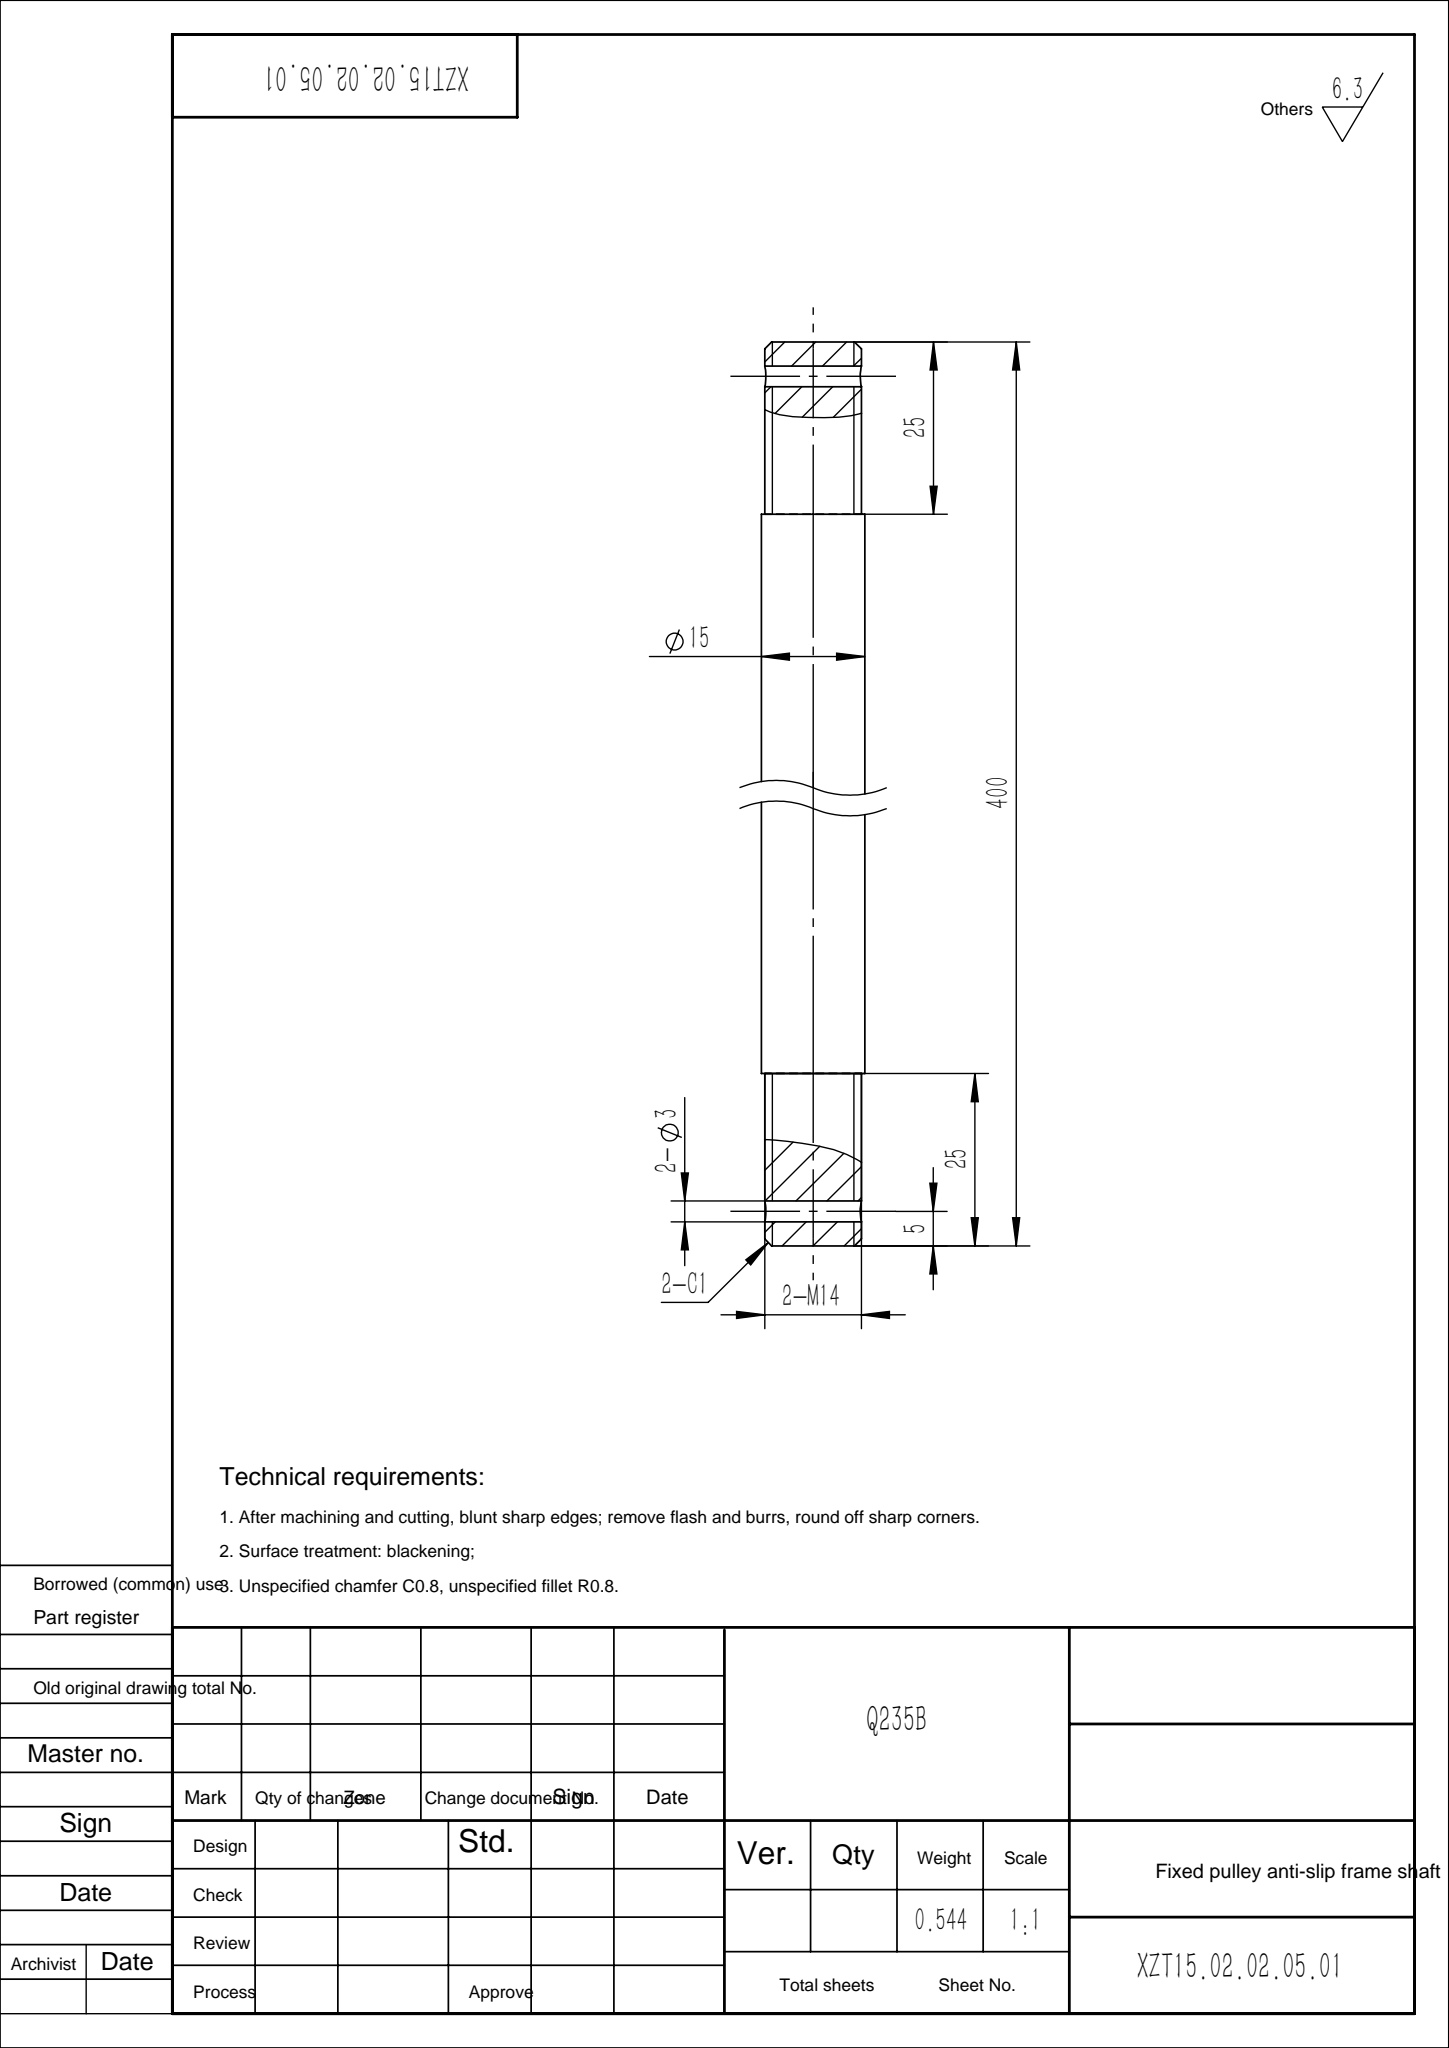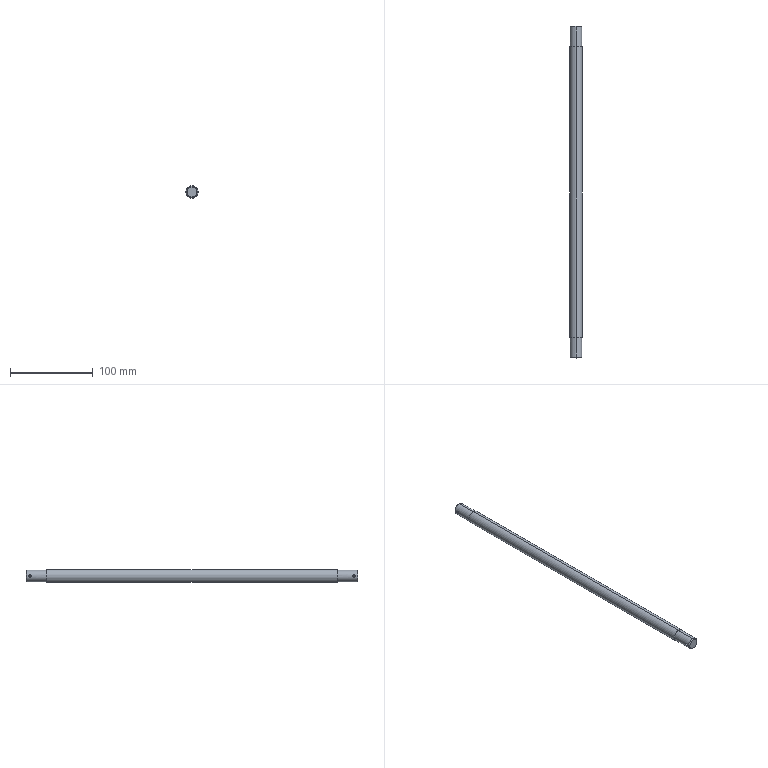Part | SolidWorks | features Chamfer 1, ICE 1, Revolution 1 | 1 solid | 18 faces | box 15 x 400 x 15 mm | volume 69308 mm3 | cylinder 10 | cone 4 | plane 4 | commonest cylinder face diameters 3 x4 14 x4 15 x2
STEP:
#1=CARTESIAN_POINT('',(-6.837,5.,1.5));
#2=VERTEX_POINT('',#1);
#3=CARTESIAN_POINT('',(-6.837,5.,-1.5));
#4=VERTEX_POINT('',#3);
#5=CARTESIAN_POINT('',(-6.837,5.,1.5));
#6=CARTESIAN_POINT('',(-6.837,4.804,1.5));
#7=CARTESIAN_POINT('',(-6.846,4.606,1.46));
#8=CARTESIAN_POINT('',(-6.877,4.245,1.311));
#9=CARTESIAN_POINT('',(-6.898,4.078,1.199));
#10=CARTESIAN_POINT('',(-6.93,3.871,0.9922));
#11=CARTESIAN_POINT('',(-6.94,3.808,0.9153));
#12=CARTESIAN_POINT('',(-6.96,3.699,0.753));
#13=CARTESIAN_POINT('',(-6.969,3.653,0.667));
#14=CARTESIAN_POINT('',(-6.991,3.539,0.3938));
#15=CARTESIAN_POINT('',(-7.,3.5,0.1987));
#16=CARTESIAN_POINT('',(-7.,3.5,-0.09833));
#17=CARTESIAN_POINT('',(-6.998,3.51,-0.1959));
#18=CARTESIAN_POINT('',(-6.99,3.548,-0.3882));
#19=CARTESIAN_POINT('',(-6.984,3.577,-0.4839));
#20=CARTESIAN_POINT('',(-6.961,3.689,-0.7556));
#21=CARTESIAN_POINT('',(-6.94,3.801,-0.9222));
#22=CARTESIAN_POINT('',(-6.898,4.076,-1.198));
#23=CARTESIAN_POINT('',(-6.877,4.243,-1.31));
#24=CARTESIAN_POINT('',(-6.846,4.604,-1.46));
#25=CARTESIAN_POINT('',(-6.837,4.801,-1.5));
#26=CARTESIAN_POINT('',(-6.837,5.,-1.5));
#27=B_SPLINE_CURVE_WITH_KNOTS('',3,(#5,#6,#7,#8,#9,#10,#11,#12,#13,#14,#15,#16,#17,#18,#19,#20,#21,#22,#23,#24,#25,#26),.UNSPECIFIED.,.F.,.F.,(4,2,2,2,2,2,2,2,2,2,4),(0.004703,0.005291,0.005879,0.006173,0.006467,0.007054,0.007348,0.007642,0.00823,0.008818,0.009405),.UNSPECIFIED.);
#28=EDGE_CURVE('',#2,#4,#27,.T.);
#29=ORIENTED_EDGE('',*,*,#28,.F.);
#30=CARTESIAN_POINT('',(6.837,5.,1.5));
#31=VERTEX_POINT('',#30);
#32=CARTESIAN_POINT('',(-7.5,5.,1.5));
#33=DIRECTION('',(1.,0.,0.));
#34=VECTOR('',#33,1000.);
#35=LINE('',#32,#34);
#36=EDGE_CURVE('',#2,#31,#35,.T.);
#37=ORIENTED_EDGE('',*,*,#36,.T.);
#38=CARTESIAN_POINT('',(6.837,5.,-1.5));
#39=VERTEX_POINT('',#38);
#40=CARTESIAN_POINT('',(6.837,5.,-1.5));
#41=CARTESIAN_POINT('',(6.837,4.901,-1.5));
#42=CARTESIAN_POINT('',(6.84,4.803,-1.49));
#43=CARTESIAN_POINT('',(6.848,4.611,-1.452));
#44=CARTESIAN_POINT('',(6.854,4.515,-1.423));
#45=CARTESIAN_POINT('',(6.869,4.334,-1.348));
#46=CARTESIAN_POINT('',(6.878,4.248,-1.301));
#47=CARTESIAN_POINT('',(6.898,4.085,-1.193));
#48=CARTESIAN_POINT('',(6.909,4.008,-1.129));
#49=CARTESIAN_POINT('',(6.94,3.801,-0.9225));
#50=CARTESIAN_POINT('',(6.961,3.69,-0.7555));
#51=CARTESIAN_POINT('',(6.991,3.54,-0.3947));
#52=CARTESIAN_POINT('',(7.,3.5,-0.1969));
#53=CARTESIAN_POINT('',(7.,3.5,0.09757));
#54=CARTESIAN_POINT('',(6.998,3.51,0.1973));
#55=CARTESIAN_POINT('',(6.99,3.548,0.3899));
#56=CARTESIAN_POINT('',(6.984,3.577,0.4836));
#57=CARTESIAN_POINT('',(6.961,3.69,0.7565));
#58=CARTESIAN_POINT('',(6.941,3.8,0.9216));
#59=CARTESIAN_POINT('',(6.908,4.009,1.13));
#60=CARTESIAN_POINT('',(6.898,4.085,1.192));
#61=CARTESIAN_POINT('',(6.878,4.247,1.301));
#62=CARTESIAN_POINT('',(6.869,4.335,1.348));
#63=CARTESIAN_POINT('',(6.854,4.516,1.423));
#64=CARTESIAN_POINT('',(6.848,4.609,1.452));
#65=CARTESIAN_POINT('',(6.84,4.802,1.49));
#66=CARTESIAN_POINT('',(6.837,4.902,1.5));
#67=CARTESIAN_POINT('',(6.837,5.,1.5));
#68=B_SPLINE_CURVE_WITH_KNOTS('',3,(#40,#41,#42,#43,#44,#45,#46,#47,#48,#49,#50,#51,#52,#53,#54,#55,#56,#57,#58,#59,#60,#61,#62,#63,#64,#65,#66,#67),.UNSPECIFIED.,.F.,.F.,(4,2,2,2,2,2,2,2,2,2,2,2,2,4),(0.,0.000294,0.0005879,0.0008819,0.001176,0.001764,0.002352,0.002646,0.00294,0.003527,0.003821,0.004115,0.004409,0.004703),.UNSPECIFIED.);
#69=EDGE_CURVE('',#39,#31,#68,.T.);
#70=ORIENTED_EDGE('',*,*,#69,.F.);
#71=CARTESIAN_POINT('',(-7.5,5.,-1.5));
#72=DIRECTION('',(1.,0.,0.));
#73=VECTOR('',#72,1000.);
#74=LINE('',#71,#73);
#75=EDGE_CURVE('',#4,#39,#74,.T.);
#76=ORIENTED_EDGE('',*,*,#75,.F.);
#77=EDGE_LOOP('',(#29,#37,#70,#76));
#78=FACE_OUTER_BOUND('',#77,.T.);
#79=CARTESIAN_POINT('',(-7.5,5.,0.));
#80=DIRECTION('',(1.,0.,0.));
#81=DIRECTION('',(0.,0.,-1.));
#82=AXIS2_PLACEMENT_3D('',#79,#80,#81);
#83=CYLINDRICAL_SURFACE('',#82,1.5);
#84=ADVANCED_FACE('',(#78),#83,.F.);
#85=CARTESIAN_POINT('',(-6.837,395.,1.5));
#86=VERTEX_POINT('',#85);
#87=CARTESIAN_POINT('',(-6.837,395.,-1.5));
#88=VERTEX_POINT('',#87);
#89=CARTESIAN_POINT('',(-6.837,395.,1.5));
#90=CARTESIAN_POINT('',(-6.837,394.804,1.5));
#91=CARTESIAN_POINT('',(-6.846,394.606,1.46));
#92=CARTESIAN_POINT('',(-6.877,394.245,1.311));
#93=CARTESIAN_POINT('',(-6.898,394.078,1.199));
#94=CARTESIAN_POINT('',(-6.93,393.871,0.9922));
#95=CARTESIAN_POINT('',(-6.94,393.808,0.9153));
#96=CARTESIAN_POINT('',(-6.96,393.699,0.753));
#97=CARTESIAN_POINT('',(-6.969,393.653,0.667));
#98=CARTESIAN_POINT('',(-6.991,393.539,0.3938));
#99=CARTESIAN_POINT('',(-7.,393.5,0.1987));
#100=CARTESIAN_POINT('',(-7.,393.5,-0.09833));
#101=CARTESIAN_POINT('',(-6.998,393.51,-0.1959));
#102=CARTESIAN_POINT('',(-6.99,393.548,-0.3882));
#103=CARTESIAN_POINT('',(-6.984,393.577,-0.4839));
#104=CARTESIAN_POINT('',(-6.961,393.689,-0.7556));
#105=CARTESIAN_POINT('',(-6.94,393.801,-0.9222));
#106=CARTESIAN_POINT('',(-6.898,394.076,-1.198));
#107=CARTESIAN_POINT('',(-6.877,394.243,-1.31));
#108=CARTESIAN_POINT('',(-6.846,394.604,-1.46));
#109=CARTESIAN_POINT('',(-6.837,394.801,-1.5));
#110=CARTESIAN_POINT('',(-6.837,395.,-1.5));
#111=B_SPLINE_CURVE_WITH_KNOTS('',3,(#89,#90,#91,#92,#93,#94,#95,#96,#97,#98,#99,#100,#101,#102,#103,#104,#105,#106,#107,#108,#109,#110),.UNSPECIFIED.,.F.,.F.,(4,2,2,2,2,2,2,2,2,2,4),(0.004703,0.005291,0.005879,0.006173,0.006467,0.007054,0.007348,0.007642,0.00823,0.008818,0.009405),.UNSPECIFIED.);
#112=EDGE_CURVE('',#86,#88,#111,.T.);
#113=ORIENTED_EDGE('',*,*,#112,.F.);
#114=CARTESIAN_POINT('',(6.837,395.,1.5));
#115=VERTEX_POINT('',#114);
#116=CARTESIAN_POINT('',(-7.5,395.,1.5));
#117=DIRECTION('',(1.,0.,0.));
#118=VECTOR('',#117,1000.);
#119=LINE('',#116,#118);
#120=EDGE_CURVE('',#86,#115,#119,.T.);
#121=ORIENTED_EDGE('',*,*,#120,.T.);
#122=CARTESIAN_POINT('',(6.837,395.,-1.5));
#123=VERTEX_POINT('',#122);
#124=CARTESIAN_POINT('',(6.837,395.,-1.5));
#125=CARTESIAN_POINT('',(6.837,394.901,-1.5));
#126=CARTESIAN_POINT('',(6.84,394.803,-1.49));
#127=CARTESIAN_POINT('',(6.848,394.611,-1.452));
#128=CARTESIAN_POINT('',(6.854,394.515,-1.423));
#129=CARTESIAN_POINT('',(6.869,394.334,-1.348));
#130=CARTESIAN_POINT('',(6.878,394.248,-1.301));
#131=CARTESIAN_POINT('',(6.898,394.085,-1.193));
#132=CARTESIAN_POINT('',(6.909,394.008,-1.129));
#133=CARTESIAN_POINT('',(6.94,393.801,-0.9225));
#134=CARTESIAN_POINT('',(6.961,393.69,-0.7555));
#135=CARTESIAN_POINT('',(6.991,393.54,-0.3947));
#136=CARTESIAN_POINT('',(7.,393.5,-0.1969));
#137=CARTESIAN_POINT('',(7.,393.5,0.09757));
#138=CARTESIAN_POINT('',(6.998,393.51,0.1973));
#139=CARTESIAN_POINT('',(6.99,393.548,0.3899));
#140=CARTESIAN_POINT('',(6.984,393.577,0.4836));
#141=CARTESIAN_POINT('',(6.961,393.69,0.7565));
#142=CARTESIAN_POINT('',(6.941,393.8,0.9216));
#143=CARTESIAN_POINT('',(6.908,394.009,1.13));
#144=CARTESIAN_POINT('',(6.898,394.085,1.192));
#145=CARTESIAN_POINT('',(6.878,394.247,1.301));
#146=CARTESIAN_POINT('',(6.869,394.335,1.348));
#147=CARTESIAN_POINT('',(6.854,394.516,1.423));
#148=CARTESIAN_POINT('',(6.848,394.609,1.452));
#149=CARTESIAN_POINT('',(6.84,394.802,1.49));
#150=CARTESIAN_POINT('',(6.837,394.902,1.5));
#151=CARTESIAN_POINT('',(6.837,395.,1.5));
#152=B_SPLINE_CURVE_WITH_KNOTS('',3,(#124,#125,#126,#127,#128,#129,#130,#131,#132,#133,#134,#135,#136,#137,#138,#139,#140,#141,#142,#143,#144,#145,#146,#147,#148,#149,#150,#151),.UNSPECIFIED.,.F.,.F.,(4,2,2,2,2,2,2,2,2,2,2,2,2,4),(0.,0.000294,0.0005879,0.0008819,0.001176,0.001764,0.002352,0.002646,0.00294,0.003527,0.003821,0.004115,0.004409,0.004703),.UNSPECIFIED.);
#153=EDGE_CURVE('',#123,#115,#152,.T.);
#154=ORIENTED_EDGE('',*,*,#153,.F.);
#155=CARTESIAN_POINT('',(-7.5,395.,-1.5));
#156=DIRECTION('',(1.,0.,0.));
#157=VECTOR('',#156,1000.);
#158=LINE('',#155,#157);
#159=EDGE_CURVE('',#88,#123,#158,.T.);
#160=ORIENTED_EDGE('',*,*,#159,.F.);
#161=EDGE_LOOP('',(#113,#121,#154,#160));
#162=FACE_OUTER_BOUND('',#161,.T.);
#163=CARTESIAN_POINT('',(-7.5,395.,0.));
#164=DIRECTION('',(1.,0.,0.));
#165=DIRECTION('',(0.,0.,-1.));
#166=AXIS2_PLACEMENT_3D('',#163,#164,#165);
#167=CYLINDRICAL_SURFACE('',#166,1.5);
#168=ADVANCED_FACE('',(#162),#167,.F.);
#169=CARTESIAN_POINT('',(0.,400.,6.));
#170=VERTEX_POINT('',#169);
#171=CARTESIAN_POINT('',(0.,400.,-6.));
#172=VERTEX_POINT('',#171);
#173=CARTESIAN_POINT('',(0.,400.,0.));
#174=DIRECTION('',(0.,1.,0.));
#175=DIRECTION('',(0.,0.,-1.));
#176=AXIS2_PLACEMENT_3D('',#173,#174,#175);
#177=CIRCLE('',#176,6.);
#178=EDGE_CURVE('',#170,#172,#177,.T.);
#179=ORIENTED_EDGE('',*,*,#178,.F.);
#180=CARTESIAN_POINT('',(0.,399.,7.));
#181=VERTEX_POINT('',#180);
#182=CARTESIAN_POINT('',(0.,400.,6.));
#183=DIRECTION('',(0.,-0.7071,0.7071));
#184=VECTOR('',#183,1000.);
#185=LINE('',#182,#184);
#186=EDGE_CURVE('',#170,#181,#185,.T.);
#187=ORIENTED_EDGE('',*,*,#186,.T.);
#188=CARTESIAN_POINT('',(0.,399.,-7.));
#189=VERTEX_POINT('',#188);
#190=CARTESIAN_POINT('',(0.,399.,0.));
#191=DIRECTION('',(0.,-1.,0.));
#192=DIRECTION('',(0.,0.,-1.));
#193=AXIS2_PLACEMENT_3D('',#190,#191,#192);
#194=CIRCLE('',#193,7.);
#195=EDGE_CURVE('',#189,#181,#194,.T.);
#196=ORIENTED_EDGE('',*,*,#195,.F.);
#197=CARTESIAN_POINT('',(0.,400.,-6.));
#198=DIRECTION('',(0.,-0.7071,-0.7071));
#199=VECTOR('',#198,1000.);
#200=LINE('',#197,#199);
#201=EDGE_CURVE('',#172,#189,#200,.T.);
#202=ORIENTED_EDGE('',*,*,#201,.F.);
#203=EDGE_LOOP('',(#179,#187,#196,#202));
#204=FACE_OUTER_BOUND('',#203,.T.);
#205=CARTESIAN_POINT('',(0.,400.,0.));
#206=DIRECTION('',(0.,-1.,0.));
#207=DIRECTION('',(0.,0.,-1.));
#208=AXIS2_PLACEMENT_3D('',#205,#206,#207);
#209=CONICAL_SURFACE('',#208,6.,0.7854);
#210=ADVANCED_FACE('',(#204),#209,.T.);
#211=CARTESIAN_POINT('',(0.,0.,-6.));
#212=VERTEX_POINT('',#211);
#213=CARTESIAN_POINT('',(0.,0.,6.));
#214=VERTEX_POINT('',#213);
#215=CARTESIAN_POINT('',(0.,0.,0.));
#216=DIRECTION('',(0.,-1.,0.));
#217=DIRECTION('',(0.,0.,1.));
#218=AXIS2_PLACEMENT_3D('',#215,#216,#217);
#219=CIRCLE('',#218,6.);
#220=EDGE_CURVE('',#212,#214,#219,.T.);
#221=ORIENTED_EDGE('',*,*,#220,.F.);
#222=CARTESIAN_POINT('',(0.,1.,-7.));
#223=VERTEX_POINT('',#222);
#224=CARTESIAN_POINT('',(0.,1.,-7.));
#225=DIRECTION('',(0.,0.7071,-0.7071));
#226=VECTOR('',#225,1000.);
#227=LINE('',#224,#226);
#228=EDGE_CURVE('',#212,#223,#227,.T.);
#229=ORIENTED_EDGE('',*,*,#228,.T.);
#230=CARTESIAN_POINT('',(0.,1.,7.));
#231=VERTEX_POINT('',#230);
#232=CARTESIAN_POINT('',(0.,1.,0.));
#233=DIRECTION('',(0.,1.,0.));
#234=DIRECTION('',(0.,0.,1.));
#235=AXIS2_PLACEMENT_3D('',#232,#233,#234);
#236=CIRCLE('',#235,7.);
#237=EDGE_CURVE('',#231,#223,#236,.T.);
#238=ORIENTED_EDGE('',*,*,#237,.F.);
#239=CARTESIAN_POINT('',(0.,1.,7.));
#240=DIRECTION('',(0.,0.7071,0.7071));
#241=VECTOR('',#240,1000.);
#242=LINE('',#239,#241);
#243=EDGE_CURVE('',#214,#231,#242,.T.);
#244=ORIENTED_EDGE('',*,*,#243,.F.);
#245=EDGE_LOOP('',(#221,#229,#238,#244));
#246=FACE_OUTER_BOUND('',#245,.T.);
#247=CARTESIAN_POINT('',(0.,1.,0.));
#248=DIRECTION('',(0.,1.,0.));
#249=DIRECTION('',(0.,0.,1.));
#250=AXIS2_PLACEMENT_3D('',#247,#248,#249);
#251=CONICAL_SURFACE('',#250,7.,0.7854);
#252=ADVANCED_FACE('',(#246),#251,.T.);
#253=ORIENTED_EDGE('',*,*,#153,.T.);
#254=CARTESIAN_POINT('',(6.837,395.,1.5));
#255=CARTESIAN_POINT('',(6.837,395.196,1.5));
#256=CARTESIAN_POINT('',(6.846,395.394,1.46));
#257=CARTESIAN_POINT('',(6.877,395.755,1.311));
#258=CARTESIAN_POINT('',(6.898,395.922,1.199));
#259=CARTESIAN_POINT('',(6.93,396.129,0.9922));
#260=CARTESIAN_POINT('',(6.94,396.192,0.9153));
#261=CARTESIAN_POINT('',(6.96,396.301,0.753));
#262=CARTESIAN_POINT('',(6.969,396.347,0.667));
#263=CARTESIAN_POINT('',(6.991,396.461,0.3938));
#264=CARTESIAN_POINT('',(7.,396.5,0.1987));
#265=CARTESIAN_POINT('',(7.,396.5,-0.09833));
#266=CARTESIAN_POINT('',(6.998,396.49,-0.1959));
#267=CARTESIAN_POINT('',(6.99,396.452,-0.3882));
#268=CARTESIAN_POINT('',(6.984,396.423,-0.4839));
#269=CARTESIAN_POINT('',(6.961,396.311,-0.7556));
#270=CARTESIAN_POINT('',(6.94,396.199,-0.9222));
#271=CARTESIAN_POINT('',(6.898,395.924,-1.198));
#272=CARTESIAN_POINT('',(6.877,395.757,-1.31));
#273=CARTESIAN_POINT('',(6.846,395.396,-1.46));
#274=CARTESIAN_POINT('',(6.837,395.199,-1.5));
#275=CARTESIAN_POINT('',(6.837,395.,-1.5));
#276=B_SPLINE_CURVE_WITH_KNOTS('',3,(#254,#255,#256,#257,#258,#259,#260,#261,#262,#263,#264,#265,#266,#267,#268,#269,#270,#271,#272,#273,#274,#275),.UNSPECIFIED.,.F.,.F.,(4,2,2,2,2,2,2,2,2,2,4),(0.004703,0.005291,0.005879,0.006173,0.006467,0.007054,0.007348,0.007642,0.00823,0.008818,0.009405),.UNSPECIFIED.);
#277=EDGE_CURVE('',#115,#123,#276,.T.);
#278=ORIENTED_EDGE('',*,*,#277,.T.);
#279=EDGE_LOOP('',(#253,#278));
#280=FACE_BOUND('',#279,.T.);
#281=CARTESIAN_POINT('',(0.,375.,7.));
#282=VERTEX_POINT('',#281);
#283=CARTESIAN_POINT('',(0.,375.,-7.));
#284=VERTEX_POINT('',#283);
#285=CARTESIAN_POINT('',(0.,375.,0.));
#286=DIRECTION('',(0.,1.,0.));
#287=DIRECTION('',(0.,0.,1.));
#288=AXIS2_PLACEMENT_3D('',#285,#286,#287);
#289=CIRCLE('',#288,7.);
#290=EDGE_CURVE('',#282,#284,#289,.T.);
#291=ORIENTED_EDGE('',*,*,#290,.T.);
#292=CARTESIAN_POINT('',(0.,0.,-7.));
#293=DIRECTION('',(0.,1.,0.));
#294=VECTOR('',#293,1000.);
#295=LINE('',#292,#294);
#296=EDGE_CURVE('',#284,#189,#295,.T.);
#297=ORIENTED_EDGE('',*,*,#296,.T.);
#298=ORIENTED_EDGE('',*,*,#195,.T.);
#299=CARTESIAN_POINT('',(0.,0.,7.));
#300=DIRECTION('',(0.,1.,0.));
#301=VECTOR('',#300,1000.);
#302=LINE('',#299,#301);
#303=EDGE_CURVE('',#282,#181,#302,.T.);
#304=ORIENTED_EDGE('',*,*,#303,.F.);
#305=EDGE_LOOP('',(#291,#297,#298,#304));
#306=FACE_OUTER_BOUND('',#305,.T.);
#307=CARTESIAN_POINT('',(0.,0.,0.));
#308=DIRECTION('',(0.,1.,0.));
#309=DIRECTION('',(0.,0.,1.));
#310=AXIS2_PLACEMENT_3D('',#307,#308,#309);
#311=CYLINDRICAL_SURFACE('',#310,7.);
#312=ADVANCED_FACE('',(#280,#306),#311,.T.);
#313=CARTESIAN_POINT('',(0.,25.,7.5));
#314=VERTEX_POINT('',#313);
#315=CARTESIAN_POINT('',(0.,25.,-7.5));
#316=VERTEX_POINT('',#315);
#317=CARTESIAN_POINT('',(0.,25.,0.));
#318=DIRECTION('',(0.,1.,0.));
#319=DIRECTION('',(0.,0.,1.));
#320=AXIS2_PLACEMENT_3D('',#317,#318,#319);
#321=CIRCLE('',#320,7.5);
#322=EDGE_CURVE('',#314,#316,#321,.T.);
#323=ORIENTED_EDGE('',*,*,#322,.T.);
#324=CARTESIAN_POINT('',(0.,375.,-7.5));
#325=VERTEX_POINT('',#324);
#326=CARTESIAN_POINT('',(0.,0.,-7.5));
#327=DIRECTION('',(0.,1.,0.));
#328=VECTOR('',#327,1000.);
#329=LINE('',#326,#328);
#330=EDGE_CURVE('',#316,#325,#329,.T.);
#331=ORIENTED_EDGE('',*,*,#330,.T.);
#332=CARTESIAN_POINT('',(0.,375.,7.5));
#333=VERTEX_POINT('',#332);
#334=CARTESIAN_POINT('',(0.,375.,0.));
#335=DIRECTION('',(0.,1.,0.));
#336=DIRECTION('',(0.,0.,1.));
#337=AXIS2_PLACEMENT_3D('',#334,#335,#336);
#338=CIRCLE('',#337,7.5);
#339=EDGE_CURVE('',#333,#325,#338,.T.);
#340=ORIENTED_EDGE('',*,*,#339,.F.);
#341=CARTESIAN_POINT('',(0.,0.,7.5));
#342=DIRECTION('',(0.,1.,0.));
#343=VECTOR('',#342,1000.);
#344=LINE('',#341,#343);
#345=EDGE_CURVE('',#314,#333,#344,.T.);
#346=ORIENTED_EDGE('',*,*,#345,.F.);
#347=EDGE_LOOP('',(#323,#331,#340,#346));
#348=FACE_OUTER_BOUND('',#347,.T.);
#349=CARTESIAN_POINT('',(0.,0.,0.));
#350=DIRECTION('',(0.,1.,0.));
#351=DIRECTION('',(0.,0.,1.));
#352=AXIS2_PLACEMENT_3D('',#349,#350,#351);
#353=CYLINDRICAL_SURFACE('',#352,7.5);
#354=ADVANCED_FACE('',(#348),#353,.T.);
#355=ORIENTED_EDGE('',*,*,#69,.T.);
#356=CARTESIAN_POINT('',(6.837,5.,1.5));
#357=CARTESIAN_POINT('',(6.837,5.196,1.5));
#358=CARTESIAN_POINT('',(6.846,5.394,1.46));
#359=CARTESIAN_POINT('',(6.877,5.755,1.311));
#360=CARTESIAN_POINT('',(6.898,5.922,1.199));
#361=CARTESIAN_POINT('',(6.93,6.129,0.9922));
#362=CARTESIAN_POINT('',(6.94,6.192,0.9153));
#363=CARTESIAN_POINT('',(6.96,6.301,0.753));
#364=CARTESIAN_POINT('',(6.969,6.347,0.667));
#365=CARTESIAN_POINT('',(6.991,6.461,0.3938));
#366=CARTESIAN_POINT('',(7.,6.5,0.1987));
#367=CARTESIAN_POINT('',(7.,6.5,-0.09833));
#368=CARTESIAN_POINT('',(6.998,6.49,-0.1959));
#369=CARTESIAN_POINT('',(6.99,6.452,-0.3882));
#370=CARTESIAN_POINT('',(6.984,6.423,-0.4839));
#371=CARTESIAN_POINT('',(6.961,6.311,-0.7556));
#372=CARTESIAN_POINT('',(6.94,6.199,-0.9222));
#373=CARTESIAN_POINT('',(6.898,5.924,-1.198));
#374=CARTESIAN_POINT('',(6.877,5.757,-1.31));
#375=CARTESIAN_POINT('',(6.846,5.396,-1.46));
#376=CARTESIAN_POINT('',(6.837,5.199,-1.5));
#377=CARTESIAN_POINT('',(6.837,5.,-1.5));
#378=B_SPLINE_CURVE_WITH_KNOTS('',3,(#356,#357,#358,#359,#360,#361,#362,#363,#364,#365,#366,#367,#368,#369,#370,#371,#372,#373,#374,#375,#376,#377),.UNSPECIFIED.,.F.,.F.,(4,2,2,2,2,2,2,2,2,2,4),(0.004703,0.005291,0.005879,0.006173,0.006467,0.007054,0.007348,0.007642,0.00823,0.008818,0.009405),.UNSPECIFIED.);
#379=EDGE_CURVE('',#31,#39,#378,.T.);
#380=ORIENTED_EDGE('',*,*,#379,.T.);
#381=EDGE_LOOP('',(#355,#380));
#382=FACE_BOUND('',#381,.T.);
#383=ORIENTED_EDGE('',*,*,#237,.T.);
#384=CARTESIAN_POINT('',(0.,25.,-7.));
#385=VERTEX_POINT('',#384);
#386=CARTESIAN_POINT('',(0.,0.,-7.));
#387=DIRECTION('',(0.,1.,0.));
#388=VECTOR('',#387,1000.);
#389=LINE('',#386,#388);
#390=EDGE_CURVE('',#223,#385,#389,.T.);
#391=ORIENTED_EDGE('',*,*,#390,.T.);
#392=CARTESIAN_POINT('',(0.,25.,7.));
#393=VERTEX_POINT('',#392);
#394=CARTESIAN_POINT('',(0.,25.,0.));
#395=DIRECTION('',(0.,1.,0.));
#396=DIRECTION('',(0.,0.,1.));
#397=AXIS2_PLACEMENT_3D('',#394,#395,#396);
#398=CIRCLE('',#397,7.);
#399=EDGE_CURVE('',#393,#385,#398,.T.);
#400=ORIENTED_EDGE('',*,*,#399,.F.);
#401=CARTESIAN_POINT('',(0.,0.,7.));
#402=DIRECTION('',(0.,1.,0.));
#403=VECTOR('',#402,1000.);
#404=LINE('',#401,#403);
#405=EDGE_CURVE('',#231,#393,#404,.T.);
#406=ORIENTED_EDGE('',*,*,#405,.F.);
#407=EDGE_LOOP('',(#383,#391,#400,#406));
#408=FACE_OUTER_BOUND('',#407,.T.);
#409=CARTESIAN_POINT('',(0.,0.,0.));
#410=DIRECTION('',(0.,1.,0.));
#411=DIRECTION('',(0.,0.,1.));
#412=AXIS2_PLACEMENT_3D('',#409,#410,#411);
#413=CYLINDRICAL_SURFACE('',#412,7.);
#414=ADVANCED_FACE('',(#382,#408),#413,.T.);
#415=CARTESIAN_POINT('',(0.,0.,0.));
#416=DIRECTION('',(0.,-1.,0.));
#417=DIRECTION('',(0.,0.,1.));
#418=AXIS2_PLACEMENT_3D('',#415,#416,#417);
#419=CIRCLE('',#418,6.);
#420=EDGE_CURVE('',#214,#212,#419,.T.);
#421=ORIENTED_EDGE('',*,*,#420,.T.);
#422=ORIENTED_EDGE('',*,*,#220,.T.);
#423=EDGE_LOOP('',(#421,#422));
#424=FACE_OUTER_BOUND('',#423,.T.);
#425=CARTESIAN_POINT('',(0.,0.,0.));
#426=DIRECTION('',(0.,1.,0.));
#427=DIRECTION('',(0.,0.,1.));
#428=AXIS2_PLACEMENT_3D('',#425,#426,#427);
#429=PLANE('',#428);
#430=ADVANCED_FACE('',(#424),#429,.F.);
#431=ORIENTED_EDGE('',*,*,#390,.F.);
#432=CARTESIAN_POINT('',(0.,1.,0.));
#433=DIRECTION('',(0.,1.,0.));
#434=DIRECTION('',(0.,0.,1.));
#435=AXIS2_PLACEMENT_3D('',#432,#433,#434);
#436=CIRCLE('',#435,7.);
#437=EDGE_CURVE('',#223,#231,#436,.T.);
#438=ORIENTED_EDGE('',*,*,#437,.T.);
#439=ORIENTED_EDGE('',*,*,#405,.T.);
#440=CARTESIAN_POINT('',(0.,25.,0.));
#441=DIRECTION('',(0.,1.,0.));
#442=DIRECTION('',(0.,0.,1.));
#443=AXIS2_PLACEMENT_3D('',#440,#441,#442);
#444=CIRCLE('',#443,7.);
#445=EDGE_CURVE('',#385,#393,#444,.T.);
#446=ORIENTED_EDGE('',*,*,#445,.F.);
#447=EDGE_LOOP('',(#431,#438,#439,#446));
#448=FACE_OUTER_BOUND('',#447,.T.);
#449=CARTESIAN_POINT('',(-6.837,5.,-1.5));
#450=CARTESIAN_POINT('',(-6.837,5.099,-1.5));
#451=CARTESIAN_POINT('',(-6.84,5.197,-1.49));
#452=CARTESIAN_POINT('',(-6.848,5.389,-1.452));
#453=CARTESIAN_POINT('',(-6.854,5.485,-1.423));
#454=CARTESIAN_POINT('',(-6.869,5.666,-1.348));
#455=CARTESIAN_POINT('',(-6.878,5.752,-1.301));
#456=CARTESIAN_POINT('',(-6.898,5.915,-1.193));
#457=CARTESIAN_POINT('',(-6.909,5.992,-1.129));
#458=CARTESIAN_POINT('',(-6.94,6.199,-0.9225));
#459=CARTESIAN_POINT('',(-6.961,6.31,-0.7555));
#460=CARTESIAN_POINT('',(-6.991,6.46,-0.3947));
#461=CARTESIAN_POINT('',(-7.,6.5,-0.1969));
#462=CARTESIAN_POINT('',(-7.,6.5,0.09757));
#463=CARTESIAN_POINT('',(-6.998,6.49,0.1973));
#464=CARTESIAN_POINT('',(-6.99,6.452,0.3899));
#465=CARTESIAN_POINT('',(-6.984,6.423,0.4836));
#466=CARTESIAN_POINT('',(-6.961,6.31,0.7565));
#467=CARTESIAN_POINT('',(-6.941,6.2,0.9216));
#468=CARTESIAN_POINT('',(-6.908,5.991,1.13));
#469=CARTESIAN_POINT('',(-6.898,5.915,1.192));
#470=CARTESIAN_POINT('',(-6.878,5.753,1.301));
#471=CARTESIAN_POINT('',(-6.869,5.665,1.348));
#472=CARTESIAN_POINT('',(-6.854,5.484,1.423));
#473=CARTESIAN_POINT('',(-6.848,5.391,1.452));
#474=CARTESIAN_POINT('',(-6.84,5.198,1.49));
#475=CARTESIAN_POINT('',(-6.837,5.098,1.5));
#476=CARTESIAN_POINT('',(-6.837,5.,1.5));
#477=B_SPLINE_CURVE_WITH_KNOTS('',3,(#449,#450,#451,#452,#453,#454,#455,#456,#457,#458,#459,#460,#461,#462,#463,#464,#465,#466,#467,#468,#469,#470,#471,#472,#473,#474,#475,#476),.UNSPECIFIED.,.F.,.F.,(4,2,2,2,2,2,2,2,2,2,2,2,2,4),(0.,0.000294,0.0005879,0.0008819,0.001176,0.001764,0.002352,0.002646,0.00294,0.003527,0.003821,0.004115,0.004409,0.004703),.UNSPECIFIED.);
#478=EDGE_CURVE('',#4,#2,#477,.T.);
#479=ORIENTED_EDGE('',*,*,#478,.T.);
#480=ORIENTED_EDGE('',*,*,#28,.T.);
#481=EDGE_LOOP('',(#479,#480));
#482=FACE_BOUND('',#481,.T.);
#483=CARTESIAN_POINT('',(0.,0.,0.));
#484=DIRECTION('',(0.,1.,0.));
#485=DIRECTION('',(0.,0.,1.));
#486=AXIS2_PLACEMENT_3D('',#483,#484,#485);
#487=CYLINDRICAL_SURFACE('',#486,7.);
#488=ADVANCED_FACE('',(#448,#482),#487,.T.);
#489=ORIENTED_EDGE('',*,*,#322,.F.);
#490=CARTESIAN_POINT('',(0.,25.,0.));
#491=DIRECTION('',(0.,1.,0.));
#492=DIRECTION('',(0.,0.,1.));
#493=AXIS2_PLACEMENT_3D('',#490,#491,#492);
#494=CIRCLE('',#493,7.5);
#495=EDGE_CURVE('',#316,#314,#494,.T.);
#496=ORIENTED_EDGE('',*,*,#495,.F.);
#497=EDGE_LOOP('',(#489,#496));
#498=FACE_OUTER_BOUND('',#497,.T.);
#499=ORIENTED_EDGE('',*,*,#399,.T.);
#500=ORIENTED_EDGE('',*,*,#445,.T.);
#501=EDGE_LOOP('',(#499,#500));
#502=FACE_BOUND('',#501,.T.);
#503=CARTESIAN_POINT('',(7.,25.,0.));
#504=DIRECTION('',(0.,1.,0.));
#505=DIRECTION('',(0.,0.,1.));
#506=AXIS2_PLACEMENT_3D('',#503,#504,#505);
#507=PLANE('',#506);
#508=ADVANCED_FACE('',(#498,#502),#507,.F.);
#509=ORIENTED_EDGE('',*,*,#330,.F.);
#510=ORIENTED_EDGE('',*,*,#495,.T.);
#511=ORIENTED_EDGE('',*,*,#345,.T.);
#512=CARTESIAN_POINT('',(0.,375.,0.));
#513=DIRECTION('',(0.,1.,0.));
#514=DIRECTION('',(0.,0.,1.));
#515=AXIS2_PLACEMENT_3D('',#512,#513,#514);
#516=CIRCLE('',#515,7.5);
#517=EDGE_CURVE('',#325,#333,#516,.T.);
#518=ORIENTED_EDGE('',*,*,#517,.F.);
#519=EDGE_LOOP('',(#509,#510,#511,#518));
#520=FACE_OUTER_BOUND('',#519,.T.);
#521=CARTESIAN_POINT('',(0.,0.,0.));
#522=DIRECTION('',(0.,1.,0.));
#523=DIRECTION('',(0.,0.,1.));
#524=AXIS2_PLACEMENT_3D('',#521,#522,#523);
#525=CYLINDRICAL_SURFACE('',#524,7.5);
#526=ADVANCED_FACE('',(#520),#525,.T.);
#527=ORIENTED_EDGE('',*,*,#290,.F.);
#528=CARTESIAN_POINT('',(0.,375.,0.));
#529=DIRECTION('',(0.,1.,0.));
#530=DIRECTION('',(0.,0.,1.));
#531=AXIS2_PLACEMENT_3D('',#528,#529,#530);
#532=CIRCLE('',#531,7.);
#533=EDGE_CURVE('',#284,#282,#532,.T.);
#534=ORIENTED_EDGE('',*,*,#533,.F.);
#535=EDGE_LOOP('',(#527,#534));
#536=FACE_BOUND('',#535,.T.);
#537=ORIENTED_EDGE('',*,*,#339,.T.);
#538=ORIENTED_EDGE('',*,*,#517,.T.);
#539=EDGE_LOOP('',(#537,#538));
#540=FACE_OUTER_BOUND('',#539,.T.);
#541=CARTESIAN_POINT('',(7.5,375.,0.));
#542=DIRECTION('',(0.,-1.,0.));
#543=DIRECTION('',(0.,0.,-1.));
#544=AXIS2_PLACEMENT_3D('',#541,#542,#543);
#545=PLANE('',#544);
#546=ADVANCED_FACE('',(#536,#540),#545,.F.);
#547=ORIENTED_EDGE('',*,*,#296,.F.);
#548=ORIENTED_EDGE('',*,*,#533,.T.);
#549=ORIENTED_EDGE('',*,*,#303,.T.);
#550=CARTESIAN_POINT('',(0.,399.,0.));
#551=DIRECTION('',(0.,-1.,0.));
#552=DIRECTION('',(0.,0.,-1.));
#553=AXIS2_PLACEMENT_3D('',#550,#551,#552);
#554=CIRCLE('',#553,7.);
#555=EDGE_CURVE('',#181,#189,#554,.T.);
#556=ORIENTED_EDGE('',*,*,#555,.T.);
#557=EDGE_LOOP('',(#547,#548,#549,#556));
#558=FACE_OUTER_BOUND('',#557,.T.);
#559=CARTESIAN_POINT('',(-6.837,395.,-1.5));
#560=CARTESIAN_POINT('',(-6.837,395.099,-1.5));
#561=CARTESIAN_POINT('',(-6.84,395.197,-1.49));
#562=CARTESIAN_POINT('',(-6.848,395.389,-1.452));
#563=CARTESIAN_POINT('',(-6.854,395.485,-1.423));
#564=CARTESIAN_POINT('',(-6.869,395.666,-1.348));
#565=CARTESIAN_POINT('',(-6.878,395.752,-1.301));
#566=CARTESIAN_POINT('',(-6.898,395.915,-1.193));
#567=CARTESIAN_POINT('',(-6.909,395.992,-1.129));
#568=CARTESIAN_POINT('',(-6.94,396.199,-0.9225));
#569=CARTESIAN_POINT('',(-6.961,396.31,-0.7555));
#570=CARTESIAN_POINT('',(-6.991,396.46,-0.3947));
#571=CARTESIAN_POINT('',(-7.,396.5,-0.1969));
#572=CARTESIAN_POINT('',(-7.,396.5,0.09757));
#573=CARTESIAN_POINT('',(-6.998,396.49,0.1973));
#574=CARTESIAN_POINT('',(-6.99,396.452,0.3899));
#575=CARTESIAN_POINT('',(-6.984,396.423,0.4836));
#576=CARTESIAN_POINT('',(-6.961,396.31,0.7565));
#577=CARTESIAN_POINT('',(-6.941,396.2,0.9216));
#578=CARTESIAN_POINT('',(-6.908,395.991,1.13));
#579=CARTESIAN_POINT('',(-6.898,395.915,1.192));
#580=CARTESIAN_POINT('',(-6.878,395.753,1.301));
#581=CARTESIAN_POINT('',(-6.869,395.665,1.348));
#582=CARTESIAN_POINT('',(-6.854,395.484,1.423));
#583=CARTESIAN_POINT('',(-6.848,395.391,1.452));
#584=CARTESIAN_POINT('',(-6.84,395.198,1.49));
#585=CARTESIAN_POINT('',(-6.837,395.098,1.5));
#586=CARTESIAN_POINT('',(-6.837,395.,1.5));
#587=B_SPLINE_CURVE_WITH_KNOTS('',3,(#559,#560,#561,#562,#563,#564,#565,#566,#567,#568,#569,#570,#571,#572,#573,#574,#575,#576,#577,#578,#579,#580,#581,#582,#583,#584,#585,#586),.UNSPECIFIED.,.F.,.F.,(4,2,2,2,2,2,2,2,2,2,2,2,2,4),(0.,0.000294,0.0005879,0.0008819,0.001176,0.001764,0.002352,0.002646,0.00294,0.003527,0.003821,0.004115,0.004409,0.004703),.UNSPECIFIED.);
#588=EDGE_CURVE('',#88,#86,#587,.T.);
#589=ORIENTED_EDGE('',*,*,#588,.T.);
#590=ORIENTED_EDGE('',*,*,#112,.T.);
#591=EDGE_LOOP('',(#589,#590));
#592=FACE_BOUND('',#591,.T.);
#593=CARTESIAN_POINT('',(0.,0.,0.));
#594=DIRECTION('',(0.,1.,0.));
#595=DIRECTION('',(0.,0.,1.));
#596=AXIS2_PLACEMENT_3D('',#593,#594,#595);
#597=CYLINDRICAL_SURFACE('',#596,7.);
#598=ADVANCED_FACE('',(#558,#592),#597,.T.);
#599=CARTESIAN_POINT('',(0.,400.,0.));
#600=DIRECTION('',(0.,1.,0.));
#601=DIRECTION('',(0.,0.,-1.));
#602=AXIS2_PLACEMENT_3D('',#599,#600,#601);
#603=CIRCLE('',#602,6.);
#604=EDGE_CURVE('',#172,#170,#603,.T.);
#605=ORIENTED_EDGE('',*,*,#604,.T.);
#606=ORIENTED_EDGE('',*,*,#178,.T.);
#607=EDGE_LOOP('',(#605,#606));
#608=FACE_OUTER_BOUND('',#607,.T.);
#609=CARTESIAN_POINT('',(7.,400.,0.));
#610=DIRECTION('',(0.,-1.,0.));
#611=DIRECTION('',(0.,0.,-1.));
#612=AXIS2_PLACEMENT_3D('',#609,#610,#611);
#613=PLANE('',#612);
#614=ADVANCED_FACE('',(#608),#613,.F.);
#615=ORIENTED_EDGE('',*,*,#228,.F.);
#616=ORIENTED_EDGE('',*,*,#420,.F.);
#617=ORIENTED_EDGE('',*,*,#243,.T.);
#618=ORIENTED_EDGE('',*,*,#437,.F.);
#619=EDGE_LOOP('',(#615,#616,#617,#618));
#620=FACE_OUTER_BOUND('',#619,.T.);
#621=CARTESIAN_POINT('',(0.,1.,0.));
#622=DIRECTION('',(0.,1.,0.));
#623=DIRECTION('',(0.,0.,1.));
#624=AXIS2_PLACEMENT_3D('',#621,#622,#623);
#625=CONICAL_SURFACE('',#624,7.,0.7854);
#626=ADVANCED_FACE('',(#620),#625,.T.);
#627=ORIENTED_EDGE('',*,*,#186,.F.);
#628=ORIENTED_EDGE('',*,*,#604,.F.);
#629=ORIENTED_EDGE('',*,*,#201,.T.);
#630=ORIENTED_EDGE('',*,*,#555,.F.);
#631=EDGE_LOOP('',(#627,#628,#629,#630));
#632=FACE_OUTER_BOUND('',#631,.T.);
#633=CARTESIAN_POINT('',(0.,400.,0.));
#634=DIRECTION('',(0.,-1.,0.));
#635=DIRECTION('',(0.,0.,-1.));
#636=AXIS2_PLACEMENT_3D('',#633,#634,#635);
#637=CONICAL_SURFACE('',#636,6.,0.7854);
#638=ADVANCED_FACE('',(#632),#637,.T.);
#639=ORIENTED_EDGE('',*,*,#120,.F.);
#640=ORIENTED_EDGE('',*,*,#588,.F.);
#641=ORIENTED_EDGE('',*,*,#159,.T.);
#642=ORIENTED_EDGE('',*,*,#277,.F.);
#643=EDGE_LOOP('',(#639,#640,#641,#642));
#644=FACE_OUTER_BOUND('',#643,.T.);
#645=CARTESIAN_POINT('',(-7.5,395.,0.));
#646=DIRECTION('',(1.,0.,0.));
#647=DIRECTION('',(0.,0.,-1.));
#648=AXIS2_PLACEMENT_3D('',#645,#646,#647);
#649=CYLINDRICAL_SURFACE('',#648,1.5);
#650=ADVANCED_FACE('',(#644),#649,.F.);
#651=ORIENTED_EDGE('',*,*,#36,.F.);
#652=ORIENTED_EDGE('',*,*,#478,.F.);
#653=ORIENTED_EDGE('',*,*,#75,.T.);
#654=ORIENTED_EDGE('',*,*,#379,.F.);
#655=EDGE_LOOP('',(#651,#652,#653,#654));
#656=FACE_OUTER_BOUND('',#655,.T.);
#657=CARTESIAN_POINT('',(-7.5,5.,0.));
#658=DIRECTION('',(1.,0.,0.));
#659=DIRECTION('',(0.,0.,-1.));
#660=AXIS2_PLACEMENT_3D('',#657,#658,#659);
#661=CYLINDRICAL_SURFACE('',#660,1.5);
#662=ADVANCED_FACE('',(#656),#661,.F.);
#663=CLOSED_SHELL('',(#84,#168,#210,#252,#312,#354,#414,#430,#488,#508,#526,#546,#598,#614,#626,#638,#650,#662));
#664=MANIFOLD_SOLID_BREP('',#663);
#665=CARTESIAN_POINT('',(0.,0.,0.));
#666=DIRECTION('',(0.,0.,1.));
#667=DIRECTION('',(1.,0.,0.));
#668=AXIS2_PLACEMENT_3D('',#665,#666,#667);
#669=(LENGTH_UNIT()NAMED_UNIT(*)SI_UNIT(.MILLI.,.METRE.));
#670=UNCERTAINTY_MEASURE_WITH_UNIT(LENGTH_MEASURE(0.00001),#669,'','');
#671=(NAMED_UNIT(*)PLANE_ANGLE_UNIT()SI_UNIT($,.RADIAN.));
#672=(NAMED_UNIT(*)SI_UNIT($,.STERADIAN.)SOLID_ANGLE_UNIT());
#673=(GEOMETRIC_REPRESENTATION_CONTEXT(3)GLOBAL_UNCERTAINTY_ASSIGNED_CONTEXT((#670))GLOBAL_UNIT_ASSIGNED_CONTEXT((#669,#671,#672))REPRESENTATION_CONTEXT('',''));
#674=ADVANCED_BREP_SHAPE_REPRESENTATION('',(#664,#668),#673);